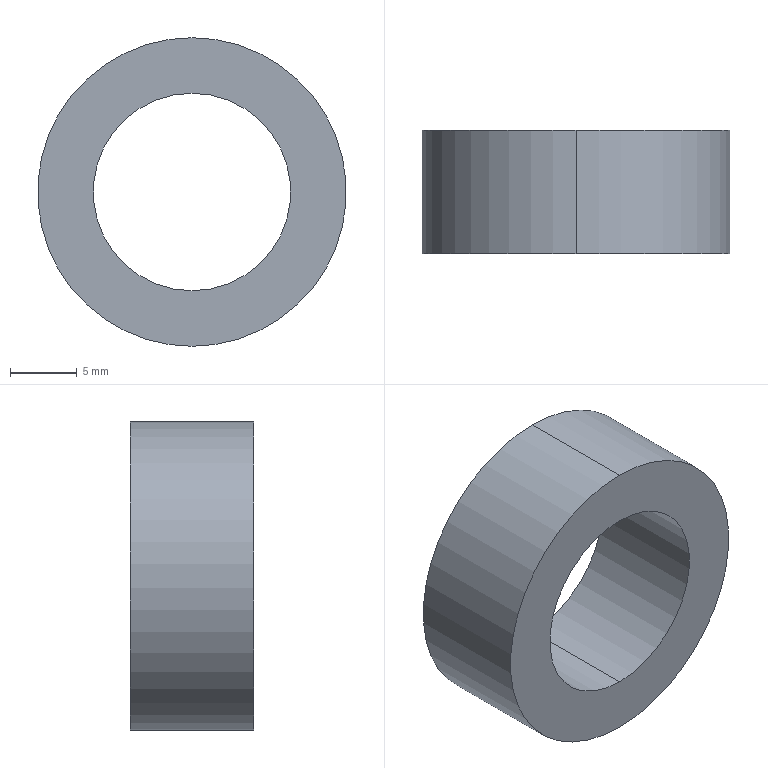Part | SolidWorks | features BaseBody 1 | 1 solid | 6 faces | box 23.077 x 9.231 x 23.077 mm | volume 2279 mm3 | cylinder 4 | plane 2 | commonest cylinder face diameters 14.769 x2 23.077 x2
STEP:
#1=CARTESIAN_POINT('',(57.247,363.731,96.154));
#2=VERTEX_POINT('',#1);
#3=CARTESIAN_POINT('',(57.247,363.731,119.231));
#4=VERTEX_POINT('',#3);
#5=CARTESIAN_POINT('',(57.247,363.731,107.692));
#6=DIRECTION('',(0.,-1.,0.));
#7=DIRECTION('',(0.,0.,-1.));
#8=AXIS2_PLACEMENT_3D('',#5,#6,#7);
#9=CIRCLE('',#8,11.538);
#10=EDGE_CURVE('',#2,#4,#9,.T.);
#11=ORIENTED_EDGE('',*,*,#10,.T.);
#12=CARTESIAN_POINT('',(57.247,354.5,119.231));
#13=VERTEX_POINT('',#12);
#14=CARTESIAN_POINT('',(57.247,363.731,119.231));
#15=DIRECTION('',(0.,-1.,0.));
#16=VECTOR('',#15,1000.);
#17=LINE('',#14,#16);
#18=EDGE_CURVE('',#4,#13,#17,.T.);
#19=ORIENTED_EDGE('',*,*,#18,.T.);
#20=CARTESIAN_POINT('',(57.247,354.5,96.154));
#21=VERTEX_POINT('',#20);
#22=CARTESIAN_POINT('',(57.247,354.5,107.692));
#23=DIRECTION('',(0.,1.,0.));
#24=DIRECTION('',(0.,0.,-1.));
#25=AXIS2_PLACEMENT_3D('',#22,#23,#24);
#26=CIRCLE('',#25,11.538);
#27=EDGE_CURVE('',#13,#21,#26,.T.);
#28=ORIENTED_EDGE('',*,*,#27,.T.);
#29=CARTESIAN_POINT('',(57.247,363.731,96.154));
#30=DIRECTION('',(0.,-1.,0.));
#31=VECTOR('',#30,1000.);
#32=LINE('',#29,#31);
#33=EDGE_CURVE('',#2,#21,#32,.T.);
#34=ORIENTED_EDGE('',*,*,#33,.F.);
#35=EDGE_LOOP('',(#11,#19,#28,#34));
#36=FACE_OUTER_BOUND('',#35,.T.);
#37=CARTESIAN_POINT('',(57.247,363.731,107.692));
#38=DIRECTION('',(0.,-1.,0.));
#39=DIRECTION('',(0.,0.,-1.));
#40=AXIS2_PLACEMENT_3D('',#37,#38,#39);
#41=CYLINDRICAL_SURFACE('',#40,11.538);
#42=ADVANCED_FACE('',(#36),#41,.T.);
#43=CARTESIAN_POINT('',(57.247,363.731,115.077));
#44=VERTEX_POINT('',#43);
#45=CARTESIAN_POINT('',(57.247,363.731,100.308));
#46=VERTEX_POINT('',#45);
#47=CARTESIAN_POINT('',(57.247,363.731,107.692));
#48=DIRECTION('',(0.,-1.,0.));
#49=DIRECTION('',(0.,0.,-1.));
#50=AXIS2_PLACEMENT_3D('',#47,#48,#49);
#51=CIRCLE('',#50,7.385);
#52=EDGE_CURVE('',#44,#46,#51,.T.);
#53=ORIENTED_EDGE('',*,*,#52,.F.);
#54=CARTESIAN_POINT('',(57.247,354.5,115.077));
#55=VERTEX_POINT('',#54);
#56=CARTESIAN_POINT('',(57.247,363.731,115.077));
#57=DIRECTION('',(0.,-1.,0.));
#58=VECTOR('',#57,1000.);
#59=LINE('',#56,#58);
#60=EDGE_CURVE('',#44,#55,#59,.T.);
#61=ORIENTED_EDGE('',*,*,#60,.T.);
#62=CARTESIAN_POINT('',(57.247,354.5,100.308));
#63=VERTEX_POINT('',#62);
#64=CARTESIAN_POINT('',(57.247,354.5,107.692));
#65=DIRECTION('',(0.,1.,0.));
#66=DIRECTION('',(0.,0.,-1.));
#67=AXIS2_PLACEMENT_3D('',#64,#65,#66);
#68=CIRCLE('',#67,7.385);
#69=EDGE_CURVE('',#63,#55,#68,.T.);
#70=ORIENTED_EDGE('',*,*,#69,.F.);
#71=CARTESIAN_POINT('',(57.247,363.731,100.308));
#72=DIRECTION('',(0.,-1.,0.));
#73=VECTOR('',#72,1000.);
#74=LINE('',#71,#73);
#75=EDGE_CURVE('',#46,#63,#74,.T.);
#76=ORIENTED_EDGE('',*,*,#75,.F.);
#77=EDGE_LOOP('',(#53,#61,#70,#76));
#78=FACE_OUTER_BOUND('',#77,.T.);
#79=CARTESIAN_POINT('',(57.247,363.731,107.692));
#80=DIRECTION('',(0.,-1.,0.));
#81=DIRECTION('',(0.,0.,-1.));
#82=AXIS2_PLACEMENT_3D('',#79,#80,#81);
#83=CYLINDRICAL_SURFACE('',#82,7.385);
#84=ADVANCED_FACE('',(#78),#83,.F.);
#85=ORIENTED_EDGE('',*,*,#18,.F.);
#86=CARTESIAN_POINT('',(57.247,363.731,107.692));
#87=DIRECTION('',(0.,-1.,0.));
#88=DIRECTION('',(0.,0.,-1.));
#89=AXIS2_PLACEMENT_3D('',#86,#87,#88);
#90=CIRCLE('',#89,11.538);
#91=EDGE_CURVE('',#4,#2,#90,.T.);
#92=ORIENTED_EDGE('',*,*,#91,.T.);
#93=ORIENTED_EDGE('',*,*,#33,.T.);
#94=CARTESIAN_POINT('',(57.247,354.5,107.692));
#95=DIRECTION('',(0.,1.,0.));
#96=DIRECTION('',(0.,0.,-1.));
#97=AXIS2_PLACEMENT_3D('',#94,#95,#96);
#98=CIRCLE('',#97,11.538);
#99=EDGE_CURVE('',#21,#13,#98,.T.);
#100=ORIENTED_EDGE('',*,*,#99,.T.);
#101=EDGE_LOOP('',(#85,#92,#93,#100));
#102=FACE_OUTER_BOUND('',#101,.T.);
#103=CARTESIAN_POINT('',(57.247,363.731,107.692));
#104=DIRECTION('',(0.,-1.,0.));
#105=DIRECTION('',(0.,0.,-1.));
#106=AXIS2_PLACEMENT_3D('',#103,#104,#105);
#107=CYLINDRICAL_SURFACE('',#106,11.538);
#108=ADVANCED_FACE('',(#102),#107,.T.);
#109=CARTESIAN_POINT('',(57.247,363.731,107.692));
#110=DIRECTION('',(0.,-1.,0.));
#111=DIRECTION('',(0.,0.,-1.));
#112=AXIS2_PLACEMENT_3D('',#109,#110,#111);
#113=CIRCLE('',#112,7.385);
#114=EDGE_CURVE('',#46,#44,#113,.T.);
#115=ORIENTED_EDGE('',*,*,#114,.T.);
#116=ORIENTED_EDGE('',*,*,#52,.T.);
#117=EDGE_LOOP('',(#115,#116));
#118=FACE_BOUND('',#117,.T.);
#119=ORIENTED_EDGE('',*,*,#10,.F.);
#120=ORIENTED_EDGE('',*,*,#91,.F.);
#121=EDGE_LOOP('',(#119,#120));
#122=FACE_OUTER_BOUND('',#121,.T.);
#123=CARTESIAN_POINT('',(64.631,363.731,107.692));
#124=DIRECTION('',(0.,1.,0.));
#125=DIRECTION('',(0.,0.,1.));
#126=AXIS2_PLACEMENT_3D('',#123,#124,#125);
#127=PLANE('',#126);
#128=ADVANCED_FACE('',(#118,#122),#127,.T.);
#129=ORIENTED_EDGE('',*,*,#69,.T.);
#130=CARTESIAN_POINT('',(57.247,354.5,107.692));
#131=DIRECTION('',(0.,1.,0.));
#132=DIRECTION('',(0.,0.,-1.));
#133=AXIS2_PLACEMENT_3D('',#130,#131,#132);
#134=CIRCLE('',#133,7.385);
#135=EDGE_CURVE('',#55,#63,#134,.T.);
#136=ORIENTED_EDGE('',*,*,#135,.T.);
#137=EDGE_LOOP('',(#129,#136));
#138=FACE_BOUND('',#137,.T.);
#139=ORIENTED_EDGE('',*,*,#99,.F.);
#140=ORIENTED_EDGE('',*,*,#27,.F.);
#141=EDGE_LOOP('',(#139,#140));
#142=FACE_OUTER_BOUND('',#141,.T.);
#143=CARTESIAN_POINT('',(68.785,354.5,107.692));
#144=DIRECTION('',(0.,-1.,0.));
#145=DIRECTION('',(0.,0.,-1.));
#146=AXIS2_PLACEMENT_3D('',#143,#144,#145);
#147=PLANE('',#146);
#148=ADVANCED_FACE('',(#138,#142),#147,.T.);
#149=ORIENTED_EDGE('',*,*,#60,.F.);
#150=ORIENTED_EDGE('',*,*,#114,.F.);
#151=ORIENTED_EDGE('',*,*,#75,.T.);
#152=ORIENTED_EDGE('',*,*,#135,.F.);
#153=EDGE_LOOP('',(#149,#150,#151,#152));
#154=FACE_OUTER_BOUND('',#153,.T.);
#155=CARTESIAN_POINT('',(57.247,363.731,107.692));
#156=DIRECTION('',(0.,-1.,0.));
#157=DIRECTION('',(0.,0.,-1.));
#158=AXIS2_PLACEMENT_3D('',#155,#156,#157);
#159=CYLINDRICAL_SURFACE('',#158,7.385);
#160=ADVANCED_FACE('',(#154),#159,.F.);
#161=CLOSED_SHELL('',(#42,#84,#108,#128,#148,#160));
#162=MANIFOLD_SOLID_BREP('',#161);
#163=CARTESIAN_POINT('',(0.,0.,0.));
#164=DIRECTION('',(0.,0.,1.));
#165=DIRECTION('',(1.,0.,0.));
#166=AXIS2_PLACEMENT_3D('',#163,#164,#165);
#167=(LENGTH_UNIT()NAMED_UNIT(*)SI_UNIT(.MILLI.,.METRE.));
#168=UNCERTAINTY_MEASURE_WITH_UNIT(LENGTH_MEASURE(0.00001),#167,'','');
#169=(NAMED_UNIT(*)PLANE_ANGLE_UNIT()SI_UNIT($,.RADIAN.));
#170=(NAMED_UNIT(*)SI_UNIT($,.STERADIAN.)SOLID_ANGLE_UNIT());
#171=(GEOMETRIC_REPRESENTATION_CONTEXT(3)GLOBAL_UNCERTAINTY_ASSIGNED_CONTEXT((#168))GLOBAL_UNIT_ASSIGNED_CONTEXT((#167,#169,#170))REPRESENTATION_CONTEXT('',''));
#172=ADVANCED_BREP_SHAPE_REPRESENTATION('',(#162,#166),#171);